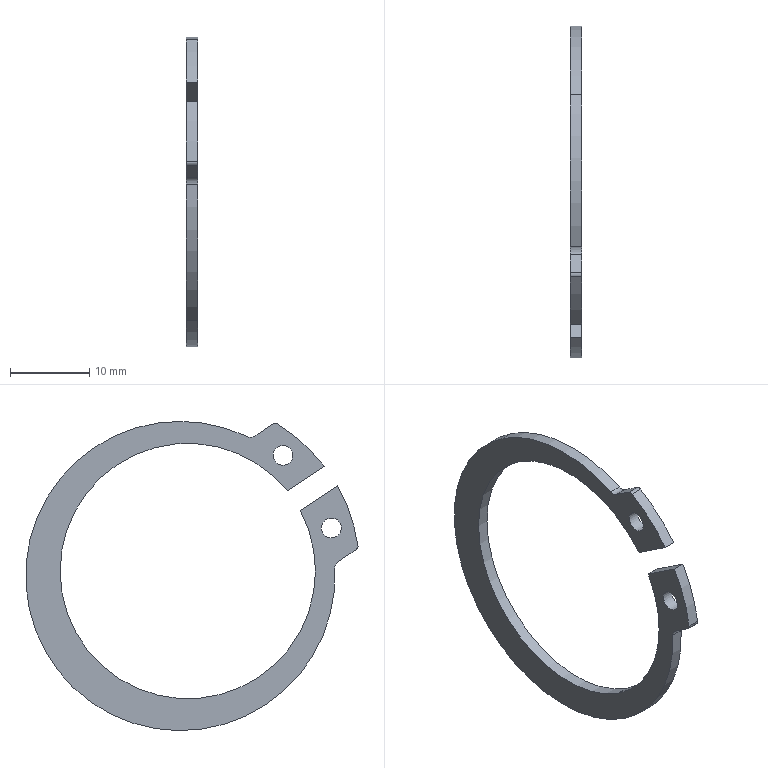Part | SolidWorks | features BaseBody 1 | 1 solid | 22 faces | box 1.5 x 41.909 x 39 mm | volume 627.923 mm3 | cylinder 16 | plane 6 | commonest cylinder face diameters 2.5 x4 32.2 x3 39 x3 1 x2 2 x2 43.4 x2
STEP:
#1=CARTESIAN_POINT('',(272.,-18.796,4.384));
#2=VERTEX_POINT('',#1);
#3=CARTESIAN_POINT('',(272.,-17.413,6.467));
#4=VERTEX_POINT('',#3);
#5=CARTESIAN_POINT('',(272.,-18.105,5.425));
#6=DIRECTION('',(-1.,0.,0.));
#7=DIRECTION('',(0.,-0.5534,-0.8329));
#8=AXIS2_PLACEMENT_3D('',#5,#6,#7);
#9=CIRCLE('',#8,1.25);
#10=EDGE_CURVE('',#2,#4,#9,.T.);
#11=ORIENTED_EDGE('',*,*,#10,.T.);
#12=CARTESIAN_POINT('',(273.5,-17.413,6.467));
#13=VERTEX_POINT('',#12);
#14=CARTESIAN_POINT('',(272.,-17.413,6.467));
#15=DIRECTION('',(1.,0.,0.));
#16=VECTOR('',#15,1000.);
#17=LINE('',#14,#16);
#18=EDGE_CURVE('',#4,#13,#17,.T.);
#19=ORIENTED_EDGE('',*,*,#18,.T.);
#20=CARTESIAN_POINT('',(273.5,-18.796,4.384));
#21=VERTEX_POINT('',#20);
#22=CARTESIAN_POINT('',(273.5,-18.105,5.425));
#23=DIRECTION('',(-1.,0.,0.));
#24=DIRECTION('',(0.,-0.5534,-0.8329));
#25=AXIS2_PLACEMENT_3D('',#22,#23,#24);
#26=CIRCLE('',#25,1.25);
#27=EDGE_CURVE('',#21,#13,#26,.T.);
#28=ORIENTED_EDGE('',*,*,#27,.F.);
#29=CARTESIAN_POINT('',(272.,-18.796,4.384));
#30=DIRECTION('',(1.,0.,0.));
#31=VECTOR('',#30,1000.);
#32=LINE('',#29,#31);
#33=EDGE_CURVE('',#2,#21,#32,.T.);
#34=ORIENTED_EDGE('',*,*,#33,.F.);
#35=EDGE_LOOP('',(#11,#19,#28,#34));
#36=FACE_OUTER_BOUND('',#35,.T.);
#37=CARTESIAN_POINT('',(272.,-18.105,5.425));
#38=DIRECTION('',(1.,0.,0.));
#39=DIRECTION('',(0.,-0.5534,-0.8329));
#40=AXIS2_PLACEMENT_3D('',#37,#38,#39);
#41=CYLINDRICAL_SURFACE('',#40,1.25);
#42=ADVANCED_FACE('',(#36),#41,.F.);
#43=CARTESIAN_POINT('',(272.,-12.709,13.546));
#44=VERTEX_POINT('',#43);
#45=CARTESIAN_POINT('',(272.,-11.326,15.629));
#46=VERTEX_POINT('',#45);
#47=CARTESIAN_POINT('',(272.,-12.017,14.588));
#48=DIRECTION('',(-1.,0.,0.));
#49=DIRECTION('',(0.,0.5534,0.8329));
#50=AXIS2_PLACEMENT_3D('',#47,#48,#49);
#51=CIRCLE('',#50,1.25);
#52=EDGE_CURVE('',#44,#46,#51,.T.);
#53=ORIENTED_EDGE('',*,*,#52,.T.);
#54=CARTESIAN_POINT('',(273.5,-11.326,15.629));
#55=VERTEX_POINT('',#54);
#56=CARTESIAN_POINT('',(272.,-11.326,15.629));
#57=DIRECTION('',(1.,0.,0.));
#58=VECTOR('',#57,1000.);
#59=LINE('',#56,#58);
#60=EDGE_CURVE('',#46,#55,#59,.T.);
#61=ORIENTED_EDGE('',*,*,#60,.T.);
#62=CARTESIAN_POINT('',(273.5,-12.709,13.546));
#63=VERTEX_POINT('',#62);
#64=CARTESIAN_POINT('',(273.5,-12.017,14.588));
#65=DIRECTION('',(-1.,0.,0.));
#66=DIRECTION('',(0.,0.5534,0.8329));
#67=AXIS2_PLACEMENT_3D('',#64,#65,#66);
#68=CIRCLE('',#67,1.25);
#69=EDGE_CURVE('',#63,#55,#68,.T.);
#70=ORIENTED_EDGE('',*,*,#69,.F.);
#71=CARTESIAN_POINT('',(272.,-12.709,13.546));
#72=DIRECTION('',(1.,0.,0.));
#73=VECTOR('',#72,1000.);
#74=LINE('',#71,#73);
#75=EDGE_CURVE('',#44,#63,#74,.T.);
#76=ORIENTED_EDGE('',*,*,#75,.F.);
#77=EDGE_LOOP('',(#53,#61,#70,#76));
#78=FACE_OUTER_BOUND('',#77,.T.);
#79=CARTESIAN_POINT('',(272.,-12.017,14.588));
#80=DIRECTION('',(1.,0.,0.));
#81=DIRECTION('',(0.,-0.5534,-0.8329));
#82=AXIS2_PLACEMENT_3D('',#79,#80,#81);
#83=CYLINDRICAL_SURFACE('',#82,1.25);
#84=ADVANCED_FACE('',(#78),#83,.F.);
#85=CARTESIAN_POINT('',(272.,11.732,15.617));
#86=VERTEX_POINT('',#85);
#87=CARTESIAN_POINT('',(272.,-9.85,-16.867));
#88=VERTEX_POINT('',#87);
#89=CARTESIAN_POINT('',(272.,0.9412,-0.6253));
#90=DIRECTION('',(-1.,0.,0.));
#91=DIRECTION('',(0.,0.5534,0.8329));
#92=AXIS2_PLACEMENT_3D('',#89,#90,#91);
#93=CIRCLE('',#92,19.5);
#94=EDGE_CURVE('',#86,#88,#93,.T.);
#95=ORIENTED_EDGE('',*,*,#94,.F.);
#96=CARTESIAN_POINT('',(273.5,11.732,15.617));
#97=VERTEX_POINT('',#96);
#98=CARTESIAN_POINT('',(272.,11.732,15.617));
#99=DIRECTION('',(1.,0.,0.));
#100=VECTOR('',#99,1000.);
#101=LINE('',#98,#100);
#102=EDGE_CURVE('',#86,#97,#101,.T.);
#103=ORIENTED_EDGE('',*,*,#102,.T.);
#104=CARTESIAN_POINT('',(273.5,-9.85,-16.867));
#105=VERTEX_POINT('',#104);
#106=CARTESIAN_POINT('',(273.5,0.9412,-0.6253));
#107=DIRECTION('',(-1.,0.,0.));
#108=DIRECTION('',(0.,0.5534,0.8329));
#109=AXIS2_PLACEMENT_3D('',#106,#107,#108);
#110=CIRCLE('',#109,19.5);
#111=EDGE_CURVE('',#97,#105,#110,.T.);
#112=ORIENTED_EDGE('',*,*,#111,.T.);
#113=CARTESIAN_POINT('',(272.,-9.85,-16.867));
#114=DIRECTION('',(1.,0.,0.));
#115=VECTOR('',#114,1000.);
#116=LINE('',#113,#115);
#117=EDGE_CURVE('',#88,#105,#116,.T.);
#118=ORIENTED_EDGE('',*,*,#117,.F.);
#119=EDGE_LOOP('',(#95,#103,#112,#118));
#120=FACE_OUTER_BOUND('',#119,.T.);
#121=CARTESIAN_POINT('',(272.,0.9412,-0.6253));
#122=DIRECTION('',(1.,0.,0.));
#123=DIRECTION('',(0.,-0.5534,-0.8329));
#124=AXIS2_PLACEMENT_3D('',#121,#122,#123);
#125=CYLINDRICAL_SURFACE('',#124,19.5);
#126=ADVANCED_FACE('',(#120),#125,.T.);
#127=CARTESIAN_POINT('',(272.,-18.536,0.3238));
#128=VERTEX_POINT('',#127);
#129=CARTESIAN_POINT('',(272.,0.9412,-0.6253));
#130=DIRECTION('',(-1.,0.,0.));
#131=DIRECTION('',(0.,0.5534,0.8329));
#132=AXIS2_PLACEMENT_3D('',#129,#130,#131);
#133=CIRCLE('',#132,19.5);
#134=EDGE_CURVE('',#88,#128,#133,.T.);
#135=ORIENTED_EDGE('',*,*,#134,.F.);
#136=ORIENTED_EDGE('',*,*,#117,.T.);
#137=CARTESIAN_POINT('',(273.5,-18.536,0.3238));
#138=VERTEX_POINT('',#137);
#139=CARTESIAN_POINT('',(273.5,0.9412,-0.6253));
#140=DIRECTION('',(-1.,0.,0.));
#141=DIRECTION('',(0.,0.5534,0.8329));
#142=AXIS2_PLACEMENT_3D('',#139,#140,#141);
#143=CIRCLE('',#142,19.5);
#144=EDGE_CURVE('',#105,#138,#143,.T.);
#145=ORIENTED_EDGE('',*,*,#144,.T.);
#146=CARTESIAN_POINT('',(272.,-18.536,0.3238));
#147=DIRECTION('',(1.,0.,0.));
#148=VECTOR('',#147,1000.);
#149=LINE('',#146,#148);
#150=EDGE_CURVE('',#128,#138,#149,.T.);
#151=ORIENTED_EDGE('',*,*,#150,.F.);
#152=EDGE_LOOP('',(#135,#136,#145,#151));
#153=FACE_OUTER_BOUND('',#152,.T.);
#154=CARTESIAN_POINT('',(272.,0.9412,-0.6253));
#155=DIRECTION('',(1.,0.,0.));
#156=DIRECTION('',(0.,-0.5534,-0.8329));
#157=AXIS2_PLACEMENT_3D('',#154,#155,#156);
#158=CYLINDRICAL_SURFACE('',#157,19.5);
#159=ADVANCED_FACE('',(#153),#158,.T.);
#160=CARTESIAN_POINT('',(272.,8.91,13.41));
#161=VERTEX_POINT('',#160);
#162=CARTESIAN_POINT('',(272.,-12.522,10.12));
#163=VERTEX_POINT('',#162);
#164=CARTESIAN_POINT('',(272.,0.,0.));
#165=DIRECTION('',(1.,0.,0.));
#166=DIRECTION('',(0.,0.5534,0.8329));
#167=AXIS2_PLACEMENT_3D('',#164,#165,#166);
#168=CIRCLE('',#167,16.1);
#169=EDGE_CURVE('',#161,#163,#168,.T.);
#170=ORIENTED_EDGE('',*,*,#169,.F.);
#171=CARTESIAN_POINT('',(273.5,8.91,13.41));
#172=VERTEX_POINT('',#171);
#173=CARTESIAN_POINT('',(272.,8.91,13.41));
#174=DIRECTION('',(1.,0.,0.));
#175=VECTOR('',#174,1000.);
#176=LINE('',#173,#175);
#177=EDGE_CURVE('',#161,#172,#176,.T.);
#178=ORIENTED_EDGE('',*,*,#177,.T.);
#179=CARTESIAN_POINT('',(273.5,-12.522,10.12));
#180=VERTEX_POINT('',#179);
#181=CARTESIAN_POINT('',(273.5,0.,0.));
#182=DIRECTION('',(1.,0.,0.));
#183=DIRECTION('',(0.,0.5534,0.8329));
#184=AXIS2_PLACEMENT_3D('',#181,#182,#183);
#185=CIRCLE('',#184,16.1);
#186=EDGE_CURVE('',#172,#180,#185,.T.);
#187=ORIENTED_EDGE('',*,*,#186,.T.);
#188=CARTESIAN_POINT('',(272.,-12.522,10.12));
#189=DIRECTION('',(1.,0.,0.));
#190=VECTOR('',#189,1000.);
#191=LINE('',#188,#190);
#192=EDGE_CURVE('',#163,#180,#191,.T.);
#193=ORIENTED_EDGE('',*,*,#192,.F.);
#194=EDGE_LOOP('',(#170,#178,#187,#193));
#195=FACE_OUTER_BOUND('',#194,.T.);
#196=CARTESIAN_POINT('',(272.,0.,0.));
#197=DIRECTION('',(1.,0.,0.));
#198=DIRECTION('',(0.,-0.5534,-0.8329));
#199=AXIS2_PLACEMENT_3D('',#196,#197,#198);
#200=CYLINDRICAL_SURFACE('',#199,16.1);
#201=ADVANCED_FACE('',(#195),#200,.F.);
#202=ORIENTED_EDGE('',*,*,#177,.F.);
#203=CARTESIAN_POINT('',(272.,-8.91,-13.41));
#204=VERTEX_POINT('',#203);
#205=CARTESIAN_POINT('',(272.,0.,0.));
#206=DIRECTION('',(1.,0.,0.));
#207=DIRECTION('',(0.,0.5534,0.8329));
#208=AXIS2_PLACEMENT_3D('',#205,#206,#207);
#209=CIRCLE('',#208,16.1);
#210=EDGE_CURVE('',#204,#161,#209,.T.);
#211=ORIENTED_EDGE('',*,*,#210,.F.);
#212=CARTESIAN_POINT('',(273.5,-8.91,-13.41));
#213=VERTEX_POINT('',#212);
#214=CARTESIAN_POINT('',(272.,-8.91,-13.41));
#215=DIRECTION('',(1.,0.,0.));
#216=VECTOR('',#215,1000.);
#217=LINE('',#214,#216);
#218=EDGE_CURVE('',#204,#213,#217,.T.);
#219=ORIENTED_EDGE('',*,*,#218,.T.);
#220=CARTESIAN_POINT('',(273.5,0.,0.));
#221=DIRECTION('',(1.,0.,0.));
#222=DIRECTION('',(0.,0.5534,0.8329));
#223=AXIS2_PLACEMENT_3D('',#220,#221,#222);
#224=CIRCLE('',#223,16.1);
#225=EDGE_CURVE('',#213,#172,#224,.T.);
#226=ORIENTED_EDGE('',*,*,#225,.T.);
#227=EDGE_LOOP('',(#202,#211,#219,#226));
#228=FACE_OUTER_BOUND('',#227,.T.);
#229=CARTESIAN_POINT('',(272.,0.,0.));
#230=DIRECTION('',(1.,0.,0.));
#231=DIRECTION('',(0.,-0.5534,-0.8329));
#232=AXIS2_PLACEMENT_3D('',#229,#230,#231);
#233=CYLINDRICAL_SURFACE('',#232,16.1);
#234=ADVANCED_FACE('',(#228),#233,.F.);
#235=ORIENTED_EDGE('',*,*,#52,.F.);
#236=CARTESIAN_POINT('',(272.,-12.017,14.588));
#237=DIRECTION('',(-1.,0.,0.));
#238=DIRECTION('',(0.,0.5534,0.8329));
#239=AXIS2_PLACEMENT_3D('',#236,#237,#238);
#240=CIRCLE('',#239,1.25);
#241=EDGE_CURVE('',#46,#44,#240,.T.);
#242=ORIENTED_EDGE('',*,*,#241,.F.);
#243=EDGE_LOOP('',(#235,#242));
#244=FACE_BOUND('',#243,.T.);
#245=CARTESIAN_POINT('',(272.,-18.981,1.205));
#246=VERTEX_POINT('',#245);
#247=CARTESIAN_POINT('',(272.,-19.535,0.3725));
#248=DIRECTION('',(1.,0.,0.));
#249=DIRECTION('',(0.,0.5534,0.8329));
#250=AXIS2_PLACEMENT_3D('',#247,#248,#249);
#251=CIRCLE('',#250,1.);
#252=EDGE_CURVE('',#128,#246,#251,.T.);
#253=ORIENTED_EDGE('',*,*,#252,.T.);
#254=CARTESIAN_POINT('',(272.,-21.245,2.709));
#255=VERTEX_POINT('',#254);
#256=CARTESIAN_POINT('',(272.,-18.981,1.205));
#257=DIRECTION('',(0.,-0.8329,0.5534));
#258=VECTOR('',#257,1000.);
#259=LINE('',#256,#258);
#260=EDGE_CURVE('',#246,#255,#259,.T.);
#261=ORIENTED_EDGE('',*,*,#260,.T.);
#262=CARTESIAN_POINT('',(272.,-21.463,3.2));
#263=VERTEX_POINT('',#262);
#264=CARTESIAN_POINT('',(272.,-20.968,3.126));
#265=DIRECTION('',(-1.,0.,0.));
#266=DIRECTION('',(0.,0.5534,0.8329));
#267=AXIS2_PLACEMENT_3D('',#264,#265,#266);
#268=CIRCLE('',#267,0.5);
#269=EDGE_CURVE('',#255,#263,#268,.T.);
#270=ORIENTED_EDGE('',*,*,#269,.T.);
#271=CARTESIAN_POINT('',(272.,-18.861,10.73));
#272=VERTEX_POINT('',#271);
#273=CARTESIAN_POINT('',(272.,0.,0.));
#274=DIRECTION('',(-1.,0.,0.));
#275=DIRECTION('',(0.,0.5534,0.8329));
#276=AXIS2_PLACEMENT_3D('',#273,#274,#275);
#277=CIRCLE('',#276,21.7);
#278=EDGE_CURVE('',#263,#272,#277,.T.);
#279=ORIENTED_EDGE('',*,*,#278,.T.);
#280=CARTESIAN_POINT('',(272.,-14.182,7.621));
#281=VERTEX_POINT('',#280);
#282=CARTESIAN_POINT('',(272.,-14.182,7.621));
#283=DIRECTION('',(0.,0.8329,-0.5534));
#284=VECTOR('',#283,1000.);
#285=LINE('',#282,#284);
#286=EDGE_CURVE('',#272,#281,#285,.T.);
#287=ORIENTED_EDGE('',*,*,#286,.T.);
#288=CARTESIAN_POINT('',(272.,0.,0.));
#289=DIRECTION('',(1.,0.,0.));
#290=DIRECTION('',(0.,0.5534,0.8329));
#291=AXIS2_PLACEMENT_3D('',#288,#289,#290);
#292=CIRCLE('',#291,16.1);
#293=EDGE_CURVE('',#281,#204,#292,.T.);
#294=ORIENTED_EDGE('',*,*,#293,.T.);
#295=ORIENTED_EDGE('',*,*,#210,.T.);
#296=ORIENTED_EDGE('',*,*,#169,.T.);
#297=CARTESIAN_POINT('',(272.,-17.201,13.229));
#298=VERTEX_POINT('',#297);
#299=CARTESIAN_POINT('',(272.,-12.522,10.12));
#300=DIRECTION('',(0.,-0.8329,0.5534));
#301=VECTOR('',#300,1000.);
#302=LINE('',#299,#301);
#303=EDGE_CURVE('',#163,#298,#302,.T.);
#304=ORIENTED_EDGE('',*,*,#303,.T.);
#305=CARTESIAN_POINT('',(272.,-11.267,18.546));
#306=VERTEX_POINT('',#305);
#307=CARTESIAN_POINT('',(272.,0.,0.));
#308=DIRECTION('',(-1.,0.,0.));
#309=DIRECTION('',(0.,0.5534,0.8329));
#310=AXIS2_PLACEMENT_3D('',#307,#308,#309);
#311=CIRCLE('',#310,21.7);
#312=EDGE_CURVE('',#298,#306,#311,.T.);
#313=ORIENTED_EDGE('',*,*,#312,.T.);
#314=CARTESIAN_POINT('',(272.,-10.731,18.535));
#315=VERTEX_POINT('',#314);
#316=CARTESIAN_POINT('',(272.,-11.007,18.119));
#317=DIRECTION('',(-1.,0.,0.));
#318=DIRECTION('',(0.,0.5534,0.8329));
#319=AXIS2_PLACEMENT_3D('',#316,#317,#318);
#320=CIRCLE('',#319,0.5);
#321=EDGE_CURVE('',#306,#315,#320,.T.);
#322=ORIENTED_EDGE('',*,*,#321,.T.);
#323=CARTESIAN_POINT('',(272.,-8.467,17.031));
#324=VERTEX_POINT('',#323);
#325=CARTESIAN_POINT('',(272.,-8.467,17.031));
#326=DIRECTION('',(0.,0.8329,-0.5534));
#327=VECTOR('',#326,1000.);
#328=LINE('',#325,#327);
#329=EDGE_CURVE('',#315,#324,#328,.T.);
#330=ORIENTED_EDGE('',*,*,#329,.T.);
#331=CARTESIAN_POINT('',(272.,-7.481,16.962));
#332=VERTEX_POINT('',#331);
#333=CARTESIAN_POINT('',(272.,-7.913,17.864));
#334=DIRECTION('',(1.,0.,0.));
#335=DIRECTION('',(0.,-0.5534,-0.8329));
#336=AXIS2_PLACEMENT_3D('',#333,#334,#335);
#337=CIRCLE('',#336,1.);
#338=EDGE_CURVE('',#324,#332,#337,.T.);
#339=ORIENTED_EDGE('',*,*,#338,.T.);
#340=CARTESIAN_POINT('',(272.,0.9412,-0.6253));
#341=DIRECTION('',(-1.,0.,0.));
#342=DIRECTION('',(0.,0.5534,0.8329));
#343=AXIS2_PLACEMENT_3D('',#340,#341,#342);
#344=CIRCLE('',#343,19.5);
#345=EDGE_CURVE('',#332,#86,#344,.T.);
#346=ORIENTED_EDGE('',*,*,#345,.T.);
#347=ORIENTED_EDGE('',*,*,#94,.T.);
#348=ORIENTED_EDGE('',*,*,#134,.T.);
#349=EDGE_LOOP('',(#253,#261,#270,#279,#287,#294,#295,#296,#304,#313,#322,#330,#339,#346,#347,#348));
#350=FACE_OUTER_BOUND('',#349,.T.);
#351=ORIENTED_EDGE('',*,*,#10,.F.);
#352=CARTESIAN_POINT('',(272.,-18.105,5.425));
#353=DIRECTION('',(-1.,0.,0.));
#354=DIRECTION('',(0.,-0.5534,-0.8329));
#355=AXIS2_PLACEMENT_3D('',#352,#353,#354);
#356=CIRCLE('',#355,1.25);
#357=EDGE_CURVE('',#4,#2,#356,.T.);
#358=ORIENTED_EDGE('',*,*,#357,.F.);
#359=EDGE_LOOP('',(#351,#358));
#360=FACE_BOUND('',#359,.T.);
#361=CARTESIAN_POINT('',(272.,-19.535,0.3725));
#362=DIRECTION('',(-1.,0.,0.));
#363=DIRECTION('',(0.,0.5534,0.8329));
#364=AXIS2_PLACEMENT_3D('',#361,#362,#363);
#365=PLANE('',#364);
#366=ADVANCED_FACE('',(#244,#350,#360),#365,.T.);
#367=ORIENTED_EDGE('',*,*,#69,.T.);
#368=CARTESIAN_POINT('',(273.5,-12.017,14.588));
#369=DIRECTION('',(-1.,0.,0.));
#370=DIRECTION('',(0.,0.5534,0.8329));
#371=AXIS2_PLACEMENT_3D('',#368,#369,#370);
#372=CIRCLE('',#371,1.25);
#373=EDGE_CURVE('',#55,#63,#372,.T.);
#374=ORIENTED_EDGE('',*,*,#373,.T.);
#375=EDGE_LOOP('',(#367,#374));
#376=FACE_BOUND('',#375,.T.);
#377=CARTESIAN_POINT('',(273.5,-18.981,1.205));
#378=VERTEX_POINT('',#377);
#379=CARTESIAN_POINT('',(273.5,-19.535,0.3725));
#380=DIRECTION('',(1.,0.,0.));
#381=DIRECTION('',(0.,0.5534,0.8329));
#382=AXIS2_PLACEMENT_3D('',#379,#380,#381);
#383=CIRCLE('',#382,1.);
#384=EDGE_CURVE('',#138,#378,#383,.T.);
#385=ORIENTED_EDGE('',*,*,#384,.F.);
#386=ORIENTED_EDGE('',*,*,#144,.F.);
#387=ORIENTED_EDGE('',*,*,#111,.F.);
#388=CARTESIAN_POINT('',(273.5,-7.481,16.962));
#389=VERTEX_POINT('',#388);
#390=CARTESIAN_POINT('',(273.5,0.9412,-0.6253));
#391=DIRECTION('',(-1.,0.,0.));
#392=DIRECTION('',(0.,0.5534,0.8329));
#393=AXIS2_PLACEMENT_3D('',#390,#391,#392);
#394=CIRCLE('',#393,19.5);
#395=EDGE_CURVE('',#389,#97,#394,.T.);
#396=ORIENTED_EDGE('',*,*,#395,.F.);
#397=CARTESIAN_POINT('',(273.5,-8.467,17.031));
#398=VERTEX_POINT('',#397);
#399=CARTESIAN_POINT('',(273.5,-7.913,17.864));
#400=DIRECTION('',(1.,0.,0.));
#401=DIRECTION('',(0.,-0.5534,-0.8329));
#402=AXIS2_PLACEMENT_3D('',#399,#400,#401);
#403=CIRCLE('',#402,1.);
#404=EDGE_CURVE('',#398,#389,#403,.T.);
#405=ORIENTED_EDGE('',*,*,#404,.F.);
#406=CARTESIAN_POINT('',(273.5,-10.731,18.535));
#407=VERTEX_POINT('',#406);
#408=CARTESIAN_POINT('',(273.5,-8.467,17.031));
#409=DIRECTION('',(0.,0.8329,-0.5534));
#410=VECTOR('',#409,1000.);
#411=LINE('',#408,#410);
#412=EDGE_CURVE('',#407,#398,#411,.T.);
#413=ORIENTED_EDGE('',*,*,#412,.F.);
#414=CARTESIAN_POINT('',(273.5,-11.267,18.546));
#415=VERTEX_POINT('',#414);
#416=CARTESIAN_POINT('',(273.5,-11.007,18.119));
#417=DIRECTION('',(-1.,0.,0.));
#418=DIRECTION('',(0.,0.5534,0.8329));
#419=AXIS2_PLACEMENT_3D('',#416,#417,#418);
#420=CIRCLE('',#419,0.5);
#421=EDGE_CURVE('',#415,#407,#420,.T.);
#422=ORIENTED_EDGE('',*,*,#421,.F.);
#423=CARTESIAN_POINT('',(273.5,-17.201,13.229));
#424=VERTEX_POINT('',#423);
#425=CARTESIAN_POINT('',(273.5,0.,0.));
#426=DIRECTION('',(-1.,0.,0.));
#427=DIRECTION('',(0.,0.5534,0.8329));
#428=AXIS2_PLACEMENT_3D('',#425,#426,#427);
#429=CIRCLE('',#428,21.7);
#430=EDGE_CURVE('',#424,#415,#429,.T.);
#431=ORIENTED_EDGE('',*,*,#430,.F.);
#432=CARTESIAN_POINT('',(273.5,-12.522,10.12));
#433=DIRECTION('',(0.,-0.8329,0.5534));
#434=VECTOR('',#433,1000.);
#435=LINE('',#432,#434);
#436=EDGE_CURVE('',#180,#424,#435,.T.);
#437=ORIENTED_EDGE('',*,*,#436,.F.);
#438=ORIENTED_EDGE('',*,*,#186,.F.);
#439=ORIENTED_EDGE('',*,*,#225,.F.);
#440=CARTESIAN_POINT('',(273.5,-14.182,7.621));
#441=VERTEX_POINT('',#440);
#442=CARTESIAN_POINT('',(273.5,0.,0.));
#443=DIRECTION('',(1.,0.,0.));
#444=DIRECTION('',(0.,0.5534,0.8329));
#445=AXIS2_PLACEMENT_3D('',#442,#443,#444);
#446=CIRCLE('',#445,16.1);
#447=EDGE_CURVE('',#441,#213,#446,.T.);
#448=ORIENTED_EDGE('',*,*,#447,.F.);
#449=CARTESIAN_POINT('',(273.5,-18.861,10.73));
#450=VERTEX_POINT('',#449);
#451=CARTESIAN_POINT('',(273.5,-14.182,7.621));
#452=DIRECTION('',(0.,0.8329,-0.5534));
#453=VECTOR('',#452,1000.);
#454=LINE('',#451,#453);
#455=EDGE_CURVE('',#450,#441,#454,.T.);
#456=ORIENTED_EDGE('',*,*,#455,.F.);
#457=CARTESIAN_POINT('',(273.5,-21.463,3.2));
#458=VERTEX_POINT('',#457);
#459=CARTESIAN_POINT('',(273.5,0.,0.));
#460=DIRECTION('',(-1.,0.,0.));
#461=DIRECTION('',(0.,0.5534,0.8329));
#462=AXIS2_PLACEMENT_3D('',#459,#460,#461);
#463=CIRCLE('',#462,21.7);
#464=EDGE_CURVE('',#458,#450,#463,.T.);
#465=ORIENTED_EDGE('',*,*,#464,.F.);
#466=CARTESIAN_POINT('',(273.5,-21.245,2.709));
#467=VERTEX_POINT('',#466);
#468=CARTESIAN_POINT('',(273.5,-20.968,3.126));
#469=DIRECTION('',(-1.,0.,0.));
#470=DIRECTION('',(0.,0.5534,0.8329));
#471=AXIS2_PLACEMENT_3D('',#468,#469,#470);
#472=CIRCLE('',#471,0.5);
#473=EDGE_CURVE('',#467,#458,#472,.T.);
#474=ORIENTED_EDGE('',*,*,#473,.F.);
#475=CARTESIAN_POINT('',(273.5,-18.981,1.205));
#476=DIRECTION('',(0.,-0.8329,0.5534));
#477=VECTOR('',#476,1000.);
#478=LINE('',#475,#477);
#479=EDGE_CURVE('',#378,#467,#478,.T.);
#480=ORIENTED_EDGE('',*,*,#479,.F.);
#481=EDGE_LOOP('',(#385,#386,#387,#396,#405,#413,#422,#431,#437,#438,#439,#448,#456,#465,#474,#480));
#482=FACE_OUTER_BOUND('',#481,.T.);
#483=ORIENTED_EDGE('',*,*,#27,.T.);
#484=CARTESIAN_POINT('',(273.5,-18.105,5.425));
#485=DIRECTION('',(-1.,0.,0.));
#486=DIRECTION('',(0.,-0.5534,-0.8329));
#487=AXIS2_PLACEMENT_3D('',#484,#485,#486);
#488=CIRCLE('',#487,1.25);
#489=EDGE_CURVE('',#13,#21,#488,.T.);
#490=ORIENTED_EDGE('',*,*,#489,.T.);
#491=EDGE_LOOP('',(#483,#490));
#492=FACE_BOUND('',#491,.T.);
#493=CARTESIAN_POINT('',(273.5,-19.535,0.3725));
#494=DIRECTION('',(-1.,0.,0.));
#495=DIRECTION('',(0.,0.5534,0.8329));
#496=AXIS2_PLACEMENT_3D('',#493,#494,#495);
#497=PLANE('',#496);
#498=ADVANCED_FACE('',(#376,#482,#492),#497,.F.);
#499=ORIENTED_EDGE('',*,*,#384,.T.);
#500=CARTESIAN_POINT('',(272.,-18.981,1.205));
#501=DIRECTION('',(1.,0.,0.));
#502=VECTOR('',#501,1000.);
#503=LINE('',#500,#502);
#504=EDGE_CURVE('',#246,#378,#503,.T.);
#505=ORIENTED_EDGE('',*,*,#504,.F.);
#506=ORIENTED_EDGE('',*,*,#252,.F.);
#507=ORIENTED_EDGE('',*,*,#150,.T.);
#508=EDGE_LOOP('',(#499,#505,#506,#507));
#509=FACE_OUTER_BOUND('',#508,.T.);
#510=CARTESIAN_POINT('',(272.,-19.535,0.3725));
#511=DIRECTION('',(1.,0.,0.));
#512=DIRECTION('',(0.,-0.5534,-0.8329));
#513=AXIS2_PLACEMENT_3D('',#510,#511,#512);
#514=CYLINDRICAL_SURFACE('',#513,1.);
#515=ADVANCED_FACE('',(#509),#514,.F.);
#516=ORIENTED_EDGE('',*,*,#479,.T.);
#517=CARTESIAN_POINT('',(272.,-21.245,2.709));
#518=DIRECTION('',(1.,0.,0.));
#519=VECTOR('',#518,1000.);
#520=LINE('',#517,#519);
#521=EDGE_CURVE('',#255,#467,#520,.T.);
#522=ORIENTED_EDGE('',*,*,#521,.F.);
#523=ORIENTED_EDGE('',*,*,#260,.F.);
#524=ORIENTED_EDGE('',*,*,#504,.T.);
#525=EDGE_LOOP('',(#516,#522,#523,#524));
#526=FACE_OUTER_BOUND('',#525,.T.);
#527=CARTESIAN_POINT('',(272.,-18.981,1.205));
#528=DIRECTION('',(0.,0.5534,0.8329));
#529=DIRECTION('',(0.,0.8329,-0.5534));
#530=AXIS2_PLACEMENT_3D('',#527,#528,#529);
#531=PLANE('',#530);
#532=ADVANCED_FACE('',(#526),#531,.F.);
#533=ORIENTED_EDGE('',*,*,#473,.T.);
#534=CARTESIAN_POINT('',(272.,-21.463,3.2));
#535=DIRECTION('',(1.,0.,0.));
#536=VECTOR('',#535,1000.);
#537=LINE('',#534,#536);
#538=EDGE_CURVE('',#263,#458,#537,.T.);
#539=ORIENTED_EDGE('',*,*,#538,.F.);
#540=ORIENTED_EDGE('',*,*,#269,.F.);
#541=ORIENTED_EDGE('',*,*,#521,.T.);
#542=EDGE_LOOP('',(#533,#539,#540,#541));
#543=FACE_OUTER_BOUND('',#542,.T.);
#544=CARTESIAN_POINT('',(272.,-20.968,3.126));
#545=DIRECTION('',(1.,0.,0.));
#546=DIRECTION('',(0.,-0.5534,-0.8329));
#547=AXIS2_PLACEMENT_3D('',#544,#545,#546);
#548=CYLINDRICAL_SURFACE('',#547,0.5);
#549=ADVANCED_FACE('',(#543),#548,.T.);
#550=ORIENTED_EDGE('',*,*,#464,.T.);
#551=CARTESIAN_POINT('',(272.,-18.861,10.73));
#552=DIRECTION('',(1.,0.,0.));
#553=VECTOR('',#552,1000.);
#554=LINE('',#551,#553);
#555=EDGE_CURVE('',#272,#450,#554,.T.);
#556=ORIENTED_EDGE('',*,*,#555,.F.);
#557=ORIENTED_EDGE('',*,*,#278,.F.);
#558=ORIENTED_EDGE('',*,*,#538,.T.);
#559=EDGE_LOOP('',(#550,#556,#557,#558));
#560=FACE_OUTER_BOUND('',#559,.T.);
#561=CARTESIAN_POINT('',(272.,0.,0.));
#562=DIRECTION('',(1.,0.,0.));
#563=DIRECTION('',(0.,-0.5534,-0.8329));
#564=AXIS2_PLACEMENT_3D('',#561,#562,#563);
#565=CYLINDRICAL_SURFACE('',#564,21.7);
#566=ADVANCED_FACE('',(#560),#565,.T.);
#567=ORIENTED_EDGE('',*,*,#455,.T.);
#568=CARTESIAN_POINT('',(272.,-14.182,7.621));
#569=DIRECTION('',(1.,0.,0.));
#570=VECTOR('',#569,1000.);
#571=LINE('',#568,#570);
#572=EDGE_CURVE('',#281,#441,#571,.T.);
#573=ORIENTED_EDGE('',*,*,#572,.F.);
#574=ORIENTED_EDGE('',*,*,#286,.F.);
#575=ORIENTED_EDGE('',*,*,#555,.T.);
#576=EDGE_LOOP('',(#567,#573,#574,#575));
#577=FACE_OUTER_BOUND('',#576,.T.);
#578=CARTESIAN_POINT('',(272.,-14.182,7.621));
#579=DIRECTION('',(0.,-0.5534,-0.8329));
#580=DIRECTION('',(0.,-0.8329,0.5534));
#581=AXIS2_PLACEMENT_3D('',#578,#579,#580);
#582=PLANE('',#581);
#583=ADVANCED_FACE('',(#577),#582,.F.);
#584=ORIENTED_EDGE('',*,*,#218,.F.);
#585=ORIENTED_EDGE('',*,*,#293,.F.);
#586=ORIENTED_EDGE('',*,*,#572,.T.);
#587=ORIENTED_EDGE('',*,*,#447,.T.);
#588=EDGE_LOOP('',(#584,#585,#586,#587));
#589=FACE_OUTER_BOUND('',#588,.T.);
#590=CARTESIAN_POINT('',(272.,0.,0.));
#591=DIRECTION('',(1.,0.,0.));
#592=DIRECTION('',(0.,-0.5534,-0.8329));
#593=AXIS2_PLACEMENT_3D('',#590,#591,#592);
#594=CYLINDRICAL_SURFACE('',#593,16.1);
#595=ADVANCED_FACE('',(#589),#594,.F.);
#596=ORIENTED_EDGE('',*,*,#436,.T.);
#597=CARTESIAN_POINT('',(272.,-17.201,13.229));
#598=DIRECTION('',(1.,0.,0.));
#599=VECTOR('',#598,1000.);
#600=LINE('',#597,#599);
#601=EDGE_CURVE('',#298,#424,#600,.T.);
#602=ORIENTED_EDGE('',*,*,#601,.F.);
#603=ORIENTED_EDGE('',*,*,#303,.F.);
#604=ORIENTED_EDGE('',*,*,#192,.T.);
#605=EDGE_LOOP('',(#596,#602,#603,#604));
#606=FACE_OUTER_BOUND('',#605,.T.);
#607=CARTESIAN_POINT('',(272.,-12.522,10.12));
#608=DIRECTION('',(0.,0.5534,0.8329));
#609=DIRECTION('',(0.,0.8329,-0.5534));
#610=AXIS2_PLACEMENT_3D('',#607,#608,#609);
#611=PLANE('',#610);
#612=ADVANCED_FACE('',(#606),#611,.F.);
#613=ORIENTED_EDGE('',*,*,#430,.T.);
#614=CARTESIAN_POINT('',(272.,-11.267,18.546));
#615=DIRECTION('',(1.,0.,0.));
#616=VECTOR('',#615,1000.);
#617=LINE('',#614,#616);
#618=EDGE_CURVE('',#306,#415,#617,.T.);
#619=ORIENTED_EDGE('',*,*,#618,.F.);
#620=ORIENTED_EDGE('',*,*,#312,.F.);
#621=ORIENTED_EDGE('',*,*,#601,.T.);
#622=EDGE_LOOP('',(#613,#619,#620,#621));
#623=FACE_OUTER_BOUND('',#622,.T.);
#624=CARTESIAN_POINT('',(272.,0.,0.));
#625=DIRECTION('',(1.,0.,0.));
#626=DIRECTION('',(0.,-0.5534,-0.8329));
#627=AXIS2_PLACEMENT_3D('',#624,#625,#626);
#628=CYLINDRICAL_SURFACE('',#627,21.7);
#629=ADVANCED_FACE('',(#623),#628,.T.);
#630=ORIENTED_EDGE('',*,*,#421,.T.);
#631=CARTESIAN_POINT('',(272.,-10.731,18.535));
#632=DIRECTION('',(1.,0.,0.));
#633=VECTOR('',#632,1000.);
#634=LINE('',#631,#633);
#635=EDGE_CURVE('',#315,#407,#634,.T.);
#636=ORIENTED_EDGE('',*,*,#635,.F.);
#637=ORIENTED_EDGE('',*,*,#321,.F.);
#638=ORIENTED_EDGE('',*,*,#618,.T.);
#639=EDGE_LOOP('',(#630,#636,#637,#638));
#640=FACE_OUTER_BOUND('',#639,.T.);
#641=CARTESIAN_POINT('',(272.,-11.007,18.119));
#642=DIRECTION('',(1.,0.,0.));
#643=DIRECTION('',(0.,-0.5534,-0.8329));
#644=AXIS2_PLACEMENT_3D('',#641,#642,#643);
#645=CYLINDRICAL_SURFACE('',#644,0.5);
#646=ADVANCED_FACE('',(#640),#645,.T.);
#647=ORIENTED_EDGE('',*,*,#412,.T.);
#648=CARTESIAN_POINT('',(272.,-8.467,17.031));
#649=DIRECTION('',(1.,0.,0.));
#650=VECTOR('',#649,1000.);
#651=LINE('',#648,#650);
#652=EDGE_CURVE('',#324,#398,#651,.T.);
#653=ORIENTED_EDGE('',*,*,#652,.F.);
#654=ORIENTED_EDGE('',*,*,#329,.F.);
#655=ORIENTED_EDGE('',*,*,#635,.T.);
#656=EDGE_LOOP('',(#647,#653,#654,#655));
#657=FACE_OUTER_BOUND('',#656,.T.);
#658=CARTESIAN_POINT('',(272.,-8.467,17.031));
#659=DIRECTION('',(0.,-0.5534,-0.8329));
#660=DIRECTION('',(0.,-0.8329,0.5534));
#661=AXIS2_PLACEMENT_3D('',#658,#659,#660);
#662=PLANE('',#661);
#663=ADVANCED_FACE('',(#657),#662,.F.);
#664=ORIENTED_EDGE('',*,*,#404,.T.);
#665=CARTESIAN_POINT('',(272.,-7.481,16.962));
#666=DIRECTION('',(1.,0.,0.));
#667=VECTOR('',#666,1000.);
#668=LINE('',#665,#667);
#669=EDGE_CURVE('',#332,#389,#668,.T.);
#670=ORIENTED_EDGE('',*,*,#669,.F.);
#671=ORIENTED_EDGE('',*,*,#338,.F.);
#672=ORIENTED_EDGE('',*,*,#652,.T.);
#673=EDGE_LOOP('',(#664,#670,#671,#672));
#674=FACE_OUTER_BOUND('',#673,.T.);
#675=CARTESIAN_POINT('',(272.,-7.913,17.864));
#676=DIRECTION('',(1.,0.,0.));
#677=DIRECTION('',(0.,-0.5534,-0.8329));
#678=AXIS2_PLACEMENT_3D('',#675,#676,#677);
#679=CYLINDRICAL_SURFACE('',#678,1.);
#680=ADVANCED_FACE('',(#674),#679,.F.);
#681=ORIENTED_EDGE('',*,*,#102,.F.);
#682=ORIENTED_EDGE('',*,*,#345,.F.);
#683=ORIENTED_EDGE('',*,*,#669,.T.);
#684=ORIENTED_EDGE('',*,*,#395,.T.);
#685=EDGE_LOOP('',(#681,#682,#683,#684));
#686=FACE_OUTER_BOUND('',#685,.T.);
#687=CARTESIAN_POINT('',(272.,0.9412,-0.6253));
#688=DIRECTION('',(1.,0.,0.));
#689=DIRECTION('',(0.,-0.5534,-0.8329));
#690=AXIS2_PLACEMENT_3D('',#687,#688,#689);
#691=CYLINDRICAL_SURFACE('',#690,19.5);
#692=ADVANCED_FACE('',(#686),#691,.T.);
#693=ORIENTED_EDGE('',*,*,#60,.F.);
#694=ORIENTED_EDGE('',*,*,#241,.T.);
#695=ORIENTED_EDGE('',*,*,#75,.T.);
#696=ORIENTED_EDGE('',*,*,#373,.F.);
#697=EDGE_LOOP('',(#693,#694,#695,#696));
#698=FACE_OUTER_BOUND('',#697,.T.);
#699=CARTESIAN_POINT('',(272.,-12.017,14.588));
#700=DIRECTION('',(1.,0.,0.));
#701=DIRECTION('',(0.,-0.5534,-0.8329));
#702=AXIS2_PLACEMENT_3D('',#699,#700,#701);
#703=CYLINDRICAL_SURFACE('',#702,1.25);
#704=ADVANCED_FACE('',(#698),#703,.F.);
#705=ORIENTED_EDGE('',*,*,#18,.F.);
#706=ORIENTED_EDGE('',*,*,#357,.T.);
#707=ORIENTED_EDGE('',*,*,#33,.T.);
#708=ORIENTED_EDGE('',*,*,#489,.F.);
#709=EDGE_LOOP('',(#705,#706,#707,#708));
#710=FACE_OUTER_BOUND('',#709,.T.);
#711=CARTESIAN_POINT('',(272.,-18.105,5.425));
#712=DIRECTION('',(1.,0.,0.));
#713=DIRECTION('',(0.,-0.5534,-0.8329));
#714=AXIS2_PLACEMENT_3D('',#711,#712,#713);
#715=CYLINDRICAL_SURFACE('',#714,1.25);
#716=ADVANCED_FACE('',(#710),#715,.F.);
#717=CLOSED_SHELL('',(#42,#84,#126,#159,#201,#234,#366,#498,#515,#532,#549,#566,#583,#595,#612,#629,#646,#663,#680,#692,#704,#716));
#718=MANIFOLD_SOLID_BREP('',#717);
#719=CARTESIAN_POINT('',(0.,0.,0.));
#720=DIRECTION('',(0.,0.,1.));
#721=DIRECTION('',(1.,0.,0.));
#722=AXIS2_PLACEMENT_3D('',#719,#720,#721);
#723=(LENGTH_UNIT()NAMED_UNIT(*)SI_UNIT(.MILLI.,.METRE.));
#724=UNCERTAINTY_MEASURE_WITH_UNIT(LENGTH_MEASURE(0.00001),#723,'','');
#725=(NAMED_UNIT(*)PLANE_ANGLE_UNIT()SI_UNIT($,.RADIAN.));
#726=(NAMED_UNIT(*)SI_UNIT($,.STERADIAN.)SOLID_ANGLE_UNIT());
#727=(GEOMETRIC_REPRESENTATION_CONTEXT(3)GLOBAL_UNCERTAINTY_ASSIGNED_CONTEXT((#724))GLOBAL_UNIT_ASSIGNED_CONTEXT((#723,#725,#726))REPRESENTATION_CONTEXT('',''));
#728=ADVANCED_BREP_SHAPE_REPRESENTATION('',(#718,#722),#727);